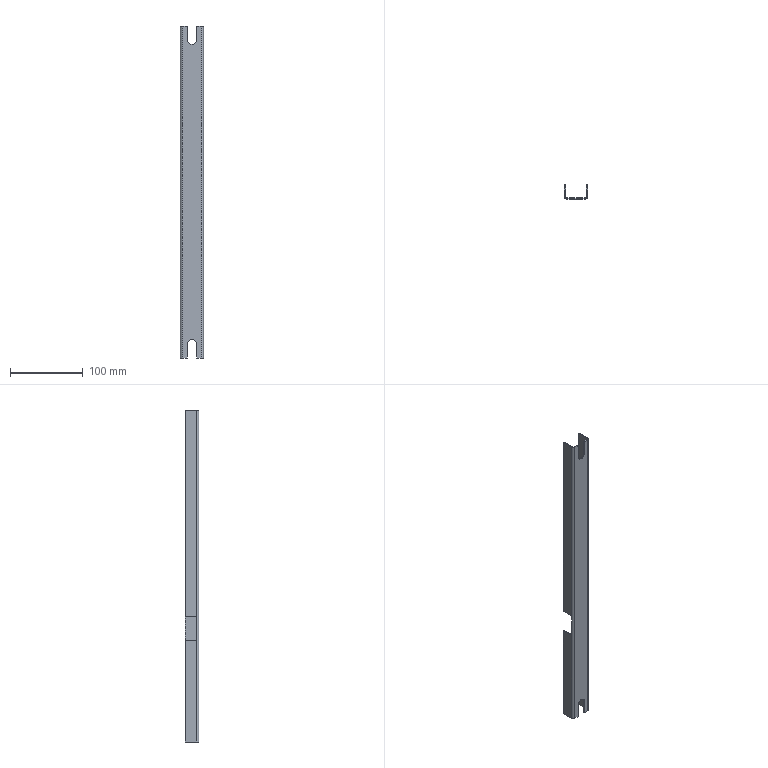Part | SolidWorks | features ICE 2, Extrusion 1, MirrorPattern 1 | 1 solid | 28 faces | box 31.75 x 19.05 x 457.2 mm | volume 42632 mm3 | plane 21 | cylinder 7 | commonest cylinder face diameters 12.7 x3 3.2 x2 6.4 x2
STEP:
#1=CARTESIAN_POINT('',(15.875,1.5,431.8));
#2=VERTEX_POINT('',#1);
#3=CARTESIAN_POINT('',(22.225,1.5,438.15));
#4=VERTEX_POINT('',#3);
#5=CARTESIAN_POINT('',(15.875,1.5,438.15));
#6=DIRECTION('',(0.,-1.,0.));
#7=DIRECTION('',(0.,0.,-1.));
#8=AXIS2_PLACEMENT_3D('',#5,#6,#7);
#9=CIRCLE('',#8,6.35);
#10=EDGE_CURVE('',#2,#4,#9,.T.);
#11=ORIENTED_EDGE('',*,*,#10,.F.);
#12=CARTESIAN_POINT('',(15.875,0.,431.8));
#13=VERTEX_POINT('',#12);
#14=CARTESIAN_POINT('',(15.875,19.05,431.8));
#15=DIRECTION('',(0.,-1.,0.));
#16=VECTOR('',#15,1000.);
#17=LINE('',#14,#16);
#18=EDGE_CURVE('',#2,#13,#17,.T.);
#19=ORIENTED_EDGE('',*,*,#18,.T.);
#20=CARTESIAN_POINT('',(22.225,0.,438.15));
#21=VERTEX_POINT('',#20);
#22=CARTESIAN_POINT('',(15.875,0.,438.15));
#23=DIRECTION('',(0.,-1.,0.));
#24=DIRECTION('',(0.,0.,-1.));
#25=AXIS2_PLACEMENT_3D('',#22,#23,#24);
#26=CIRCLE('',#25,6.35);
#27=EDGE_CURVE('',#13,#21,#26,.T.);
#28=ORIENTED_EDGE('',*,*,#27,.T.);
#29=CARTESIAN_POINT('',(22.225,19.05,438.15));
#30=DIRECTION('',(0.,-1.,0.));
#31=VECTOR('',#30,1000.);
#32=LINE('',#29,#31);
#33=EDGE_CURVE('',#4,#21,#32,.T.);
#34=ORIENTED_EDGE('',*,*,#33,.F.);
#35=EDGE_LOOP('',(#11,#19,#28,#34));
#36=FACE_OUTER_BOUND('',#35,.T.);
#37=CARTESIAN_POINT('',(15.875,19.05,438.15));
#38=DIRECTION('',(0.,-1.,0.));
#39=DIRECTION('',(0.,0.,-1.));
#40=AXIS2_PLACEMENT_3D('',#37,#38,#39);
#41=CYLINDRICAL_SURFACE('',#40,6.35);
#42=ADVANCED_FACE('',(#36),#41,.F.);
#43=CARTESIAN_POINT('',(9.525,1.5,0.));
#44=VERTEX_POINT('',#43);
#45=CARTESIAN_POINT('',(9.525,1.5,19.05));
#46=VERTEX_POINT('',#45);
#47=CARTESIAN_POINT('',(9.525,1.5,457.2));
#48=DIRECTION('',(0.,0.,1.));
#49=VECTOR('',#48,1000.);
#50=LINE('',#47,#49);
#51=EDGE_CURVE('',#44,#46,#50,.T.);
#52=ORIENTED_EDGE('',*,*,#51,.F.);
#53=CARTESIAN_POINT('',(3.1,1.5,0.));
#54=VERTEX_POINT('',#53);
#55=CARTESIAN_POINT('',(3.1,1.5,0.));
#56=DIRECTION('',(-1.,0.,0.));
#57=VECTOR('',#56,1000.);
#58=LINE('',#55,#57);
#59=EDGE_CURVE('',#44,#54,#58,.T.);
#60=ORIENTED_EDGE('',*,*,#59,.T.);
#61=CARTESIAN_POINT('',(3.1,1.5,457.2));
#62=VERTEX_POINT('',#61);
#63=CARTESIAN_POINT('',(3.1,1.5,457.2));
#64=DIRECTION('',(0.,0.,-1.));
#65=VECTOR('',#64,1000.);
#66=LINE('',#63,#65);
#67=EDGE_CURVE('',#62,#54,#66,.T.);
#68=ORIENTED_EDGE('',*,*,#67,.F.);
#69=CARTESIAN_POINT('',(9.525,1.5,457.2));
#70=VERTEX_POINT('',#69);
#71=CARTESIAN_POINT('',(3.1,1.5,457.2));
#72=DIRECTION('',(-1.,0.,0.));
#73=VECTOR('',#72,1000.);
#74=LINE('',#71,#73);
#75=EDGE_CURVE('',#70,#62,#74,.T.);
#76=ORIENTED_EDGE('',*,*,#75,.F.);
#77=CARTESIAN_POINT('',(9.525,1.5,438.15));
#78=VERTEX_POINT('',#77);
#79=CARTESIAN_POINT('',(9.525,1.5,457.2));
#80=DIRECTION('',(0.,0.,-1.));
#81=VECTOR('',#80,1000.);
#82=LINE('',#79,#81);
#83=EDGE_CURVE('',#70,#78,#82,.T.);
#84=ORIENTED_EDGE('',*,*,#83,.T.);
#85=CARTESIAN_POINT('',(15.875,1.5,438.15));
#86=DIRECTION('',(0.,-1.,0.));
#87=DIRECTION('',(0.,0.,-1.));
#88=AXIS2_PLACEMENT_3D('',#85,#86,#87);
#89=CIRCLE('',#88,6.35);
#90=EDGE_CURVE('',#78,#2,#89,.T.);
#91=ORIENTED_EDGE('',*,*,#90,.T.);
#92=ORIENTED_EDGE('',*,*,#10,.T.);
#93=CARTESIAN_POINT('',(22.225,1.5,457.2));
#94=VERTEX_POINT('',#93);
#95=CARTESIAN_POINT('',(22.225,1.5,457.2));
#96=DIRECTION('',(0.,0.,1.));
#97=VECTOR('',#96,1000.);
#98=LINE('',#95,#97);
#99=EDGE_CURVE('',#4,#94,#98,.T.);
#100=ORIENTED_EDGE('',*,*,#99,.T.);
#101=CARTESIAN_POINT('',(28.65,1.5,457.2));
#102=VERTEX_POINT('',#101);
#103=CARTESIAN_POINT('',(3.1,1.5,457.2));
#104=DIRECTION('',(-1.,0.,0.));
#105=VECTOR('',#104,1000.);
#106=LINE('',#103,#105);
#107=EDGE_CURVE('',#102,#94,#106,.T.);
#108=ORIENTED_EDGE('',*,*,#107,.F.);
#109=CARTESIAN_POINT('',(28.65,1.5,0.));
#110=VERTEX_POINT('',#109);
#111=CARTESIAN_POINT('',(28.65,1.5,457.2));
#112=DIRECTION('',(0.,0.,-1.));
#113=VECTOR('',#112,1000.);
#114=LINE('',#111,#113);
#115=EDGE_CURVE('',#102,#110,#114,.T.);
#116=ORIENTED_EDGE('',*,*,#115,.T.);
#117=CARTESIAN_POINT('',(22.225,1.5,0.));
#118=VERTEX_POINT('',#117);
#119=CARTESIAN_POINT('',(3.1,1.5,0.));
#120=DIRECTION('',(-1.,0.,0.));
#121=VECTOR('',#120,1000.);
#122=LINE('',#119,#121);
#123=EDGE_CURVE('',#110,#118,#122,.T.);
#124=ORIENTED_EDGE('',*,*,#123,.T.);
#125=CARTESIAN_POINT('',(22.225,1.5,19.05));
#126=VERTEX_POINT('',#125);
#127=CARTESIAN_POINT('',(22.225,1.5,457.2));
#128=DIRECTION('',(0.,0.,-1.));
#129=VECTOR('',#128,1000.);
#130=LINE('',#127,#129);
#131=EDGE_CURVE('',#126,#118,#130,.T.);
#132=ORIENTED_EDGE('',*,*,#131,.F.);
#133=CARTESIAN_POINT('',(15.875,1.5,19.05));
#134=DIRECTION('',(0.,1.,0.));
#135=DIRECTION('',(0.,0.,-1.));
#136=AXIS2_PLACEMENT_3D('',#133,#134,#135);
#137=CIRCLE('',#136,6.35);
#138=EDGE_CURVE('',#46,#126,#137,.T.);
#139=ORIENTED_EDGE('',*,*,#138,.F.);
#140=EDGE_LOOP('',(#52,#60,#68,#76,#84,#91,#92,#100,#108,#116,#124,#132,#139));
#141=FACE_OUTER_BOUND('',#140,.T.);
#142=CARTESIAN_POINT('',(3.1,1.5,457.2));
#143=DIRECTION('',(0.,-1.,0.));
#144=DIRECTION('',(0.,0.,-1.));
#145=AXIS2_PLACEMENT_3D('',#142,#143,#144);
#146=PLANE('',#145);
#147=ADVANCED_FACE('',(#141),#146,.F.);
#148=CARTESIAN_POINT('',(9.525,0.,0.));
#149=VERTEX_POINT('',#148);
#150=CARTESIAN_POINT('',(9.525,0.,19.05));
#151=VERTEX_POINT('',#150);
#152=CARTESIAN_POINT('',(9.525,0.,0.));
#153=DIRECTION('',(0.,0.,1.));
#154=VECTOR('',#153,1000.);
#155=LINE('',#152,#154);
#156=EDGE_CURVE('',#149,#151,#155,.T.);
#157=ORIENTED_EDGE('',*,*,#156,.T.);
#158=CARTESIAN_POINT('',(22.225,0.,19.05));
#159=VERTEX_POINT('',#158);
#160=CARTESIAN_POINT('',(15.875,0.,19.05));
#161=DIRECTION('',(0.,1.,0.));
#162=DIRECTION('',(0.,0.,1.));
#163=AXIS2_PLACEMENT_3D('',#160,#161,#162);
#164=CIRCLE('',#163,6.35);
#165=EDGE_CURVE('',#151,#159,#164,.T.);
#166=ORIENTED_EDGE('',*,*,#165,.T.);
#167=CARTESIAN_POINT('',(22.225,0.,0.));
#168=VERTEX_POINT('',#167);
#169=CARTESIAN_POINT('',(22.225,0.,0.));
#170=DIRECTION('',(0.,0.,-1.));
#171=VECTOR('',#170,1000.);
#172=LINE('',#169,#171);
#173=EDGE_CURVE('',#159,#168,#172,.T.);
#174=ORIENTED_EDGE('',*,*,#173,.T.);
#175=CARTESIAN_POINT('',(28.55,0.,0.));
#176=VERTEX_POINT('',#175);
#177=CARTESIAN_POINT('',(3.2,0.,0.));
#178=DIRECTION('',(1.,0.,0.));
#179=VECTOR('',#178,1000.);
#180=LINE('',#177,#179);
#181=EDGE_CURVE('',#168,#176,#180,.T.);
#182=ORIENTED_EDGE('',*,*,#181,.T.);
#183=CARTESIAN_POINT('',(28.55,0.,457.2));
#184=VERTEX_POINT('',#183);
#185=CARTESIAN_POINT('',(28.55,0.,457.2));
#186=DIRECTION('',(0.,0.,-1.));
#187=VECTOR('',#186,1000.);
#188=LINE('',#185,#187);
#189=EDGE_CURVE('',#184,#176,#188,.T.);
#190=ORIENTED_EDGE('',*,*,#189,.F.);
#191=CARTESIAN_POINT('',(22.225,0.,457.2));
#192=VERTEX_POINT('',#191);
#193=CARTESIAN_POINT('',(3.2,0.,457.2));
#194=DIRECTION('',(1.,0.,0.));
#195=VECTOR('',#194,1000.);
#196=LINE('',#193,#195);
#197=EDGE_CURVE('',#192,#184,#196,.T.);
#198=ORIENTED_EDGE('',*,*,#197,.F.);
#199=CARTESIAN_POINT('',(22.225,0.,457.2));
#200=DIRECTION('',(0.,0.,1.));
#201=VECTOR('',#200,1000.);
#202=LINE('',#199,#201);
#203=EDGE_CURVE('',#21,#192,#202,.T.);
#204=ORIENTED_EDGE('',*,*,#203,.F.);
#205=ORIENTED_EDGE('',*,*,#27,.F.);
#206=CARTESIAN_POINT('',(9.525,0.,438.15));
#207=VERTEX_POINT('',#206);
#208=CARTESIAN_POINT('',(15.875,0.,438.15));
#209=DIRECTION('',(0.,-1.,0.));
#210=DIRECTION('',(0.,0.,-1.));
#211=AXIS2_PLACEMENT_3D('',#208,#209,#210);
#212=CIRCLE('',#211,6.35);
#213=EDGE_CURVE('',#207,#13,#212,.T.);
#214=ORIENTED_EDGE('',*,*,#213,.F.);
#215=CARTESIAN_POINT('',(9.525,0.,457.2));
#216=VERTEX_POINT('',#215);
#217=CARTESIAN_POINT('',(9.525,0.,457.2));
#218=DIRECTION('',(0.,0.,-1.));
#219=VECTOR('',#218,1000.);
#220=LINE('',#217,#219);
#221=EDGE_CURVE('',#216,#207,#220,.T.);
#222=ORIENTED_EDGE('',*,*,#221,.F.);
#223=CARTESIAN_POINT('',(3.2,0.,457.2));
#224=VERTEX_POINT('',#223);
#225=CARTESIAN_POINT('',(3.2,0.,457.2));
#226=DIRECTION('',(1.,0.,0.));
#227=VECTOR('',#226,1000.);
#228=LINE('',#225,#227);
#229=EDGE_CURVE('',#224,#216,#228,.T.);
#230=ORIENTED_EDGE('',*,*,#229,.F.);
#231=CARTESIAN_POINT('',(3.2,0.,0.));
#232=VERTEX_POINT('',#231);
#233=CARTESIAN_POINT('',(3.2,0.,457.2));
#234=DIRECTION('',(0.,0.,-1.));
#235=VECTOR('',#234,1000.);
#236=LINE('',#233,#235);
#237=EDGE_CURVE('',#224,#232,#236,.T.);
#238=ORIENTED_EDGE('',*,*,#237,.T.);
#239=CARTESIAN_POINT('',(3.2,0.,0.));
#240=DIRECTION('',(1.,0.,0.));
#241=VECTOR('',#240,1000.);
#242=LINE('',#239,#241);
#243=EDGE_CURVE('',#232,#149,#242,.T.);
#244=ORIENTED_EDGE('',*,*,#243,.T.);
#245=EDGE_LOOP('',(#157,#166,#174,#182,#190,#198,#204,#205,#214,#222,#230,#238,#244));
#246=FACE_OUTER_BOUND('',#245,.T.);
#247=CARTESIAN_POINT('',(3.2,0.,457.2));
#248=DIRECTION('',(0.,1.,0.));
#249=DIRECTION('',(0.,0.,1.));
#250=AXIS2_PLACEMENT_3D('',#247,#248,#249);
#251=PLANE('',#250);
#252=ADVANCED_FACE('',(#246),#251,.F.);
#253=CARTESIAN_POINT('',(9.525,3.1,0.));
#254=DIRECTION('',(0.,1.,0.));
#255=VECTOR('',#254,1000.);
#256=LINE('',#253,#255);
#257=EDGE_CURVE('',#149,#44,#256,.T.);
#258=ORIENTED_EDGE('',*,*,#257,.F.);
#259=ORIENTED_EDGE('',*,*,#243,.F.);
#260=CARTESIAN_POINT('',(0.,3.2,0.));
#261=VERTEX_POINT('',#260);
#262=CARTESIAN_POINT('',(3.2,3.2,0.));
#263=DIRECTION('',(0.,0.,1.));
#264=DIRECTION('',(1.,0.,0.));
#265=AXIS2_PLACEMENT_3D('',#262,#263,#264);
#266=CIRCLE('',#265,3.2);
#267=EDGE_CURVE('',#261,#232,#266,.T.);
#268=ORIENTED_EDGE('',*,*,#267,.F.);
#269=CARTESIAN_POINT('',(0.,19.05,0.));
#270=VERTEX_POINT('',#269);
#271=CARTESIAN_POINT('',(0.,3.2,0.));
#272=DIRECTION('',(0.,-1.,0.));
#273=VECTOR('',#272,1000.);
#274=LINE('',#271,#273);
#275=EDGE_CURVE('',#270,#261,#274,.T.);
#276=ORIENTED_EDGE('',*,*,#275,.F.);
#277=CARTESIAN_POINT('',(1.5,19.05,0.));
#278=VERTEX_POINT('',#277);
#279=CARTESIAN_POINT('',(1.5,19.05,0.));
#280=DIRECTION('',(-1.,0.,0.));
#281=VECTOR('',#280,1000.);
#282=LINE('',#279,#281);
#283=EDGE_CURVE('',#278,#270,#282,.T.);
#284=ORIENTED_EDGE('',*,*,#283,.F.);
#285=CARTESIAN_POINT('',(1.5,3.1,0.));
#286=VERTEX_POINT('',#285);
#287=CARTESIAN_POINT('',(1.5,3.1,0.));
#288=DIRECTION('',(0.,1.,0.));
#289=VECTOR('',#288,1000.);
#290=LINE('',#287,#289);
#291=EDGE_CURVE('',#286,#278,#290,.T.);
#292=ORIENTED_EDGE('',*,*,#291,.F.);
#293=CARTESIAN_POINT('',(3.1,3.1,0.));
#294=DIRECTION('',(0.,0.,-1.));
#295=DIRECTION('',(-1.,0.,0.));
#296=AXIS2_PLACEMENT_3D('',#293,#294,#295);
#297=CIRCLE('',#296,1.6);
#298=EDGE_CURVE('',#54,#286,#297,.T.);
#299=ORIENTED_EDGE('',*,*,#298,.F.);
#300=ORIENTED_EDGE('',*,*,#59,.F.);
#301=EDGE_LOOP('',(#258,#259,#268,#276,#284,#292,#299,#300));
#302=FACE_OUTER_BOUND('',#301,.T.);
#303=CARTESIAN_POINT('',(28.65,3.1,0.));
#304=DIRECTION('',(0.,0.,1.));
#305=DIRECTION('',(1.,0.,0.));
#306=AXIS2_PLACEMENT_3D('',#303,#304,#305);
#307=PLANE('',#306);
#308=ADVANCED_FACE('',(#302),#307,.F.);
#309=CARTESIAN_POINT('',(22.225,3.1,0.));
#310=DIRECTION('',(0.,-1.,0.));
#311=VECTOR('',#310,1000.);
#312=LINE('',#309,#311);
#313=EDGE_CURVE('',#118,#168,#312,.T.);
#314=ORIENTED_EDGE('',*,*,#313,.F.);
#315=ORIENTED_EDGE('',*,*,#123,.F.);
#316=CARTESIAN_POINT('',(30.25,3.1,0.));
#317=VERTEX_POINT('',#316);
#318=CARTESIAN_POINT('',(28.65,3.1,0.));
#319=DIRECTION('',(0.,0.,-1.));
#320=DIRECTION('',(1.,0.,0.));
#321=AXIS2_PLACEMENT_3D('',#318,#319,#320);
#322=CIRCLE('',#321,1.6);
#323=EDGE_CURVE('',#317,#110,#322,.T.);
#324=ORIENTED_EDGE('',*,*,#323,.F.);
#325=CARTESIAN_POINT('',(30.25,19.05,0.));
#326=VERTEX_POINT('',#325);
#327=CARTESIAN_POINT('',(30.25,3.1,0.));
#328=DIRECTION('',(0.,-1.,0.));
#329=VECTOR('',#328,1000.);
#330=LINE('',#327,#329);
#331=EDGE_CURVE('',#326,#317,#330,.T.);
#332=ORIENTED_EDGE('',*,*,#331,.F.);
#333=CARTESIAN_POINT('',(31.75,19.05,0.));
#334=VERTEX_POINT('',#333);
#335=CARTESIAN_POINT('',(31.75,19.05,0.));
#336=DIRECTION('',(-1.,0.,0.));
#337=VECTOR('',#336,1000.);
#338=LINE('',#335,#337);
#339=EDGE_CURVE('',#334,#326,#338,.T.);
#340=ORIENTED_EDGE('',*,*,#339,.F.);
#341=CARTESIAN_POINT('',(31.75,3.2,0.));
#342=VERTEX_POINT('',#341);
#343=CARTESIAN_POINT('',(31.75,3.2,0.));
#344=DIRECTION('',(0.,1.,0.));
#345=VECTOR('',#344,1000.);
#346=LINE('',#343,#345);
#347=EDGE_CURVE('',#342,#334,#346,.T.);
#348=ORIENTED_EDGE('',*,*,#347,.F.);
#349=CARTESIAN_POINT('',(28.55,3.2,0.));
#350=DIRECTION('',(0.,0.,1.));
#351=DIRECTION('',(-1.,0.,0.));
#352=AXIS2_PLACEMENT_3D('',#349,#350,#351);
#353=CIRCLE('',#352,3.2);
#354=EDGE_CURVE('',#176,#342,#353,.T.);
#355=ORIENTED_EDGE('',*,*,#354,.F.);
#356=ORIENTED_EDGE('',*,*,#181,.F.);
#357=EDGE_LOOP('',(#314,#315,#324,#332,#340,#348,#355,#356));
#358=FACE_OUTER_BOUND('',#357,.T.);
#359=CARTESIAN_POINT('',(28.65,3.1,0.));
#360=DIRECTION('',(0.,0.,1.));
#361=DIRECTION('',(1.,0.,0.));
#362=AXIS2_PLACEMENT_3D('',#359,#360,#361);
#363=PLANE('',#362);
#364=ADVANCED_FACE('',(#358),#363,.F.);
#365=CARTESIAN_POINT('',(22.225,3.1,457.2));
#366=DIRECTION('',(0.,1.,0.));
#367=VECTOR('',#366,1000.);
#368=LINE('',#365,#367);
#369=EDGE_CURVE('',#192,#94,#368,.T.);
#370=ORIENTED_EDGE('',*,*,#369,.F.);
#371=ORIENTED_EDGE('',*,*,#197,.T.);
#372=CARTESIAN_POINT('',(31.75,3.2,457.2));
#373=VERTEX_POINT('',#372);
#374=CARTESIAN_POINT('',(28.55,3.2,457.2));
#375=DIRECTION('',(0.,0.,1.));
#376=DIRECTION('',(-1.,0.,0.));
#377=AXIS2_PLACEMENT_3D('',#374,#375,#376);
#378=CIRCLE('',#377,3.2);
#379=EDGE_CURVE('',#184,#373,#378,.T.);
#380=ORIENTED_EDGE('',*,*,#379,.T.);
#381=CARTESIAN_POINT('',(31.75,19.05,457.2));
#382=VERTEX_POINT('',#381);
#383=CARTESIAN_POINT('',(31.75,3.2,457.2));
#384=DIRECTION('',(0.,1.,0.));
#385=VECTOR('',#384,1000.);
#386=LINE('',#383,#385);
#387=EDGE_CURVE('',#373,#382,#386,.T.);
#388=ORIENTED_EDGE('',*,*,#387,.T.);
#389=CARTESIAN_POINT('',(30.25,19.05,457.2));
#390=VERTEX_POINT('',#389);
#391=CARTESIAN_POINT('',(31.75,19.05,457.2));
#392=DIRECTION('',(-1.,0.,0.));
#393=VECTOR('',#392,1000.);
#394=LINE('',#391,#393);
#395=EDGE_CURVE('',#382,#390,#394,.T.);
#396=ORIENTED_EDGE('',*,*,#395,.T.);
#397=CARTESIAN_POINT('',(30.25,3.1,457.2));
#398=VERTEX_POINT('',#397);
#399=CARTESIAN_POINT('',(30.25,3.1,457.2));
#400=DIRECTION('',(0.,-1.,0.));
#401=VECTOR('',#400,1000.);
#402=LINE('',#399,#401);
#403=EDGE_CURVE('',#390,#398,#402,.T.);
#404=ORIENTED_EDGE('',*,*,#403,.T.);
#405=CARTESIAN_POINT('',(28.65,3.1,457.2));
#406=DIRECTION('',(0.,0.,-1.));
#407=DIRECTION('',(1.,0.,0.));
#408=AXIS2_PLACEMENT_3D('',#405,#406,#407);
#409=CIRCLE('',#408,1.6);
#410=EDGE_CURVE('',#398,#102,#409,.T.);
#411=ORIENTED_EDGE('',*,*,#410,.T.);
#412=ORIENTED_EDGE('',*,*,#107,.T.);
#413=EDGE_LOOP('',(#370,#371,#380,#388,#396,#404,#411,#412));
#414=FACE_OUTER_BOUND('',#413,.T.);
#415=CARTESIAN_POINT('',(28.65,3.1,457.2));
#416=DIRECTION('',(0.,0.,1.));
#417=DIRECTION('',(1.,0.,0.));
#418=AXIS2_PLACEMENT_3D('',#415,#416,#417);
#419=PLANE('',#418);
#420=ADVANCED_FACE('',(#414),#419,.T.);
#421=CARTESIAN_POINT('',(1.5,19.05,457.2));
#422=VERTEX_POINT('',#421);
#423=CARTESIAN_POINT('',(1.5,19.05,172.974));
#424=VERTEX_POINT('',#423);
#425=CARTESIAN_POINT('',(1.5,19.05,457.2));
#426=DIRECTION('',(0.,0.,-1.));
#427=VECTOR('',#426,1000.);
#428=LINE('',#425,#427);
#429=EDGE_CURVE('',#422,#424,#428,.T.);
#430=ORIENTED_EDGE('',*,*,#429,.T.);
#431=CARTESIAN_POINT('',(0.,19.05,172.974));
#432=VERTEX_POINT('',#431);
#433=CARTESIAN_POINT('',(31.751,19.05,172.974));
#434=DIRECTION('',(-1.,0.,0.));
#435=VECTOR('',#434,1000.);
#436=LINE('',#433,#435);
#437=EDGE_CURVE('',#424,#432,#436,.T.);
#438=ORIENTED_EDGE('',*,*,#437,.T.);
#439=CARTESIAN_POINT('',(0.,19.05,457.2));
#440=VERTEX_POINT('',#439);
#441=CARTESIAN_POINT('',(0.,19.05,457.2));
#442=DIRECTION('',(0.,0.,-1.));
#443=VECTOR('',#442,1000.);
#444=LINE('',#441,#443);
#445=EDGE_CURVE('',#440,#432,#444,.T.);
#446=ORIENTED_EDGE('',*,*,#445,.F.);
#447=CARTESIAN_POINT('',(1.5,19.05,457.2));
#448=DIRECTION('',(-1.,0.,0.));
#449=VECTOR('',#448,1000.);
#450=LINE('',#447,#449);
#451=EDGE_CURVE('',#422,#440,#450,.T.);
#452=ORIENTED_EDGE('',*,*,#451,.F.);
#453=EDGE_LOOP('',(#430,#438,#446,#452));
#454=FACE_OUTER_BOUND('',#453,.T.);
#455=CARTESIAN_POINT('',(1.5,19.05,457.2));
#456=DIRECTION('',(0.,-1.,0.));
#457=DIRECTION('',(0.,0.,-1.));
#458=AXIS2_PLACEMENT_3D('',#455,#456,#457);
#459=PLANE('',#458);
#460=ADVANCED_FACE('',(#454),#459,.F.);
#461=ORIENTED_EDGE('',*,*,#445,.T.);
#462=CARTESIAN_POINT('',(0.,3.2,172.974));
#463=VERTEX_POINT('',#462);
#464=CARTESIAN_POINT('',(0.,19.05,172.974));
#465=DIRECTION('',(0.,1.,0.));
#466=VECTOR('',#465,1000.);
#467=LINE('',#464,#466);
#468=EDGE_CURVE('',#463,#432,#467,.T.);
#469=ORIENTED_EDGE('',*,*,#468,.F.);
#470=CARTESIAN_POINT('',(0.,3.2,457.2));
#471=VERTEX_POINT('',#470);
#472=CARTESIAN_POINT('',(0.,3.2,457.2));
#473=DIRECTION('',(0.,0.,-1.));
#474=VECTOR('',#473,1000.);
#475=LINE('',#472,#474);
#476=EDGE_CURVE('',#471,#463,#475,.T.);
#477=ORIENTED_EDGE('',*,*,#476,.F.);
#478=CARTESIAN_POINT('',(0.,3.2,457.2));
#479=DIRECTION('',(0.,-1.,0.));
#480=VECTOR('',#479,1000.);
#481=LINE('',#478,#480);
#482=EDGE_CURVE('',#440,#471,#481,.T.);
#483=ORIENTED_EDGE('',*,*,#482,.F.);
#484=EDGE_LOOP('',(#461,#469,#477,#483));
#485=FACE_OUTER_BOUND('',#484,.T.);
#486=CARTESIAN_POINT('',(0.,3.2,457.2));
#487=DIRECTION('',(1.,0.,0.));
#488=DIRECTION('',(0.,0.,-1.));
#489=AXIS2_PLACEMENT_3D('',#486,#487,#488);
#490=PLANE('',#489);
#491=ADVANCED_FACE('',(#485),#490,.F.);
#492=ORIENTED_EDGE('',*,*,#339,.T.);
#493=CARTESIAN_POINT('',(30.25,19.05,457.2));
#494=DIRECTION('',(0.,0.,-1.));
#495=VECTOR('',#494,1000.);
#496=LINE('',#493,#495);
#497=EDGE_CURVE('',#390,#326,#496,.T.);
#498=ORIENTED_EDGE('',*,*,#497,.F.);
#499=ORIENTED_EDGE('',*,*,#395,.F.);
#500=CARTESIAN_POINT('',(31.75,19.05,457.2));
#501=DIRECTION('',(0.,0.,-1.));
#502=VECTOR('',#501,1000.);
#503=LINE('',#500,#502);
#504=EDGE_CURVE('',#382,#334,#503,.T.);
#505=ORIENTED_EDGE('',*,*,#504,.T.);
#506=EDGE_LOOP('',(#492,#498,#499,#505));
#507=FACE_OUTER_BOUND('',#506,.T.);
#508=CARTESIAN_POINT('',(31.75,19.05,457.2));
#509=DIRECTION('',(0.,-1.,0.));
#510=DIRECTION('',(0.,0.,-1.));
#511=AXIS2_PLACEMENT_3D('',#508,#509,#510);
#512=PLANE('',#511);
#513=ADVANCED_FACE('',(#507),#512,.F.);
#514=ORIENTED_EDGE('',*,*,#331,.T.);
#515=CARTESIAN_POINT('',(30.25,3.1,457.2));
#516=DIRECTION('',(0.,0.,-1.));
#517=VECTOR('',#516,1000.);
#518=LINE('',#515,#517);
#519=EDGE_CURVE('',#398,#317,#518,.T.);
#520=ORIENTED_EDGE('',*,*,#519,.F.);
#521=ORIENTED_EDGE('',*,*,#403,.F.);
#522=ORIENTED_EDGE('',*,*,#497,.T.);
#523=EDGE_LOOP('',(#514,#520,#521,#522));
#524=FACE_OUTER_BOUND('',#523,.T.);
#525=CARTESIAN_POINT('',(30.25,3.1,457.2));
#526=DIRECTION('',(1.,0.,0.));
#527=DIRECTION('',(0.,1.,0.));
#528=AXIS2_PLACEMENT_3D('',#525,#526,#527);
#529=PLANE('',#528);
#530=ADVANCED_FACE('',(#524),#529,.F.);
#531=ORIENTED_EDGE('',*,*,#323,.T.);
#532=ORIENTED_EDGE('',*,*,#115,.F.);
#533=ORIENTED_EDGE('',*,*,#410,.F.);
#534=ORIENTED_EDGE('',*,*,#519,.T.);
#535=EDGE_LOOP('',(#531,#532,#533,#534));
#536=FACE_OUTER_BOUND('',#535,.T.);
#537=CARTESIAN_POINT('',(28.65,3.1,457.2));
#538=DIRECTION('',(0.,0.,-1.));
#539=DIRECTION('',(-1.,0.,0.));
#540=AXIS2_PLACEMENT_3D('',#537,#538,#539);
#541=CYLINDRICAL_SURFACE('',#540,1.6);
#542=ADVANCED_FACE('',(#536),#541,.F.);
#543=ORIENTED_EDGE('',*,*,#298,.T.);
#544=CARTESIAN_POINT('',(1.5,3.1,457.2));
#545=VERTEX_POINT('',#544);
#546=CARTESIAN_POINT('',(1.5,3.1,457.2));
#547=DIRECTION('',(0.,0.,-1.));
#548=VECTOR('',#547,1000.);
#549=LINE('',#546,#548);
#550=EDGE_CURVE('',#545,#286,#549,.T.);
#551=ORIENTED_EDGE('',*,*,#550,.F.);
#552=CARTESIAN_POINT('',(3.1,3.1,457.2));
#553=DIRECTION('',(0.,0.,-1.));
#554=DIRECTION('',(-1.,0.,0.));
#555=AXIS2_PLACEMENT_3D('',#552,#553,#554);
#556=CIRCLE('',#555,1.6);
#557=EDGE_CURVE('',#62,#545,#556,.T.);
#558=ORIENTED_EDGE('',*,*,#557,.F.);
#559=ORIENTED_EDGE('',*,*,#67,.T.);
#560=EDGE_LOOP('',(#543,#551,#558,#559));
#561=FACE_OUTER_BOUND('',#560,.T.);
#562=CARTESIAN_POINT('',(3.1,3.1,457.2));
#563=DIRECTION('',(0.,0.,-1.));
#564=DIRECTION('',(-1.,0.,0.));
#565=AXIS2_PLACEMENT_3D('',#562,#563,#564);
#566=CYLINDRICAL_SURFACE('',#565,1.6);
#567=ADVANCED_FACE('',(#561),#566,.F.);
#568=CARTESIAN_POINT('',(1.5,3.2,172.974));
#569=VERTEX_POINT('',#568);
#570=CARTESIAN_POINT('',(1.5,3.2,139.7));
#571=VERTEX_POINT('',#570);
#572=CARTESIAN_POINT('',(1.5,3.2,172.974));
#573=DIRECTION('',(0.,0.,-1.));
#574=VECTOR('',#573,1000.);
#575=LINE('',#572,#574);
#576=EDGE_CURVE('',#569,#571,#575,.T.);
#577=ORIENTED_EDGE('',*,*,#576,.F.);
#578=CARTESIAN_POINT('',(1.5,19.05,172.974));
#579=DIRECTION('',(0.,-1.,0.));
#580=VECTOR('',#579,1000.);
#581=LINE('',#578,#580);
#582=EDGE_CURVE('',#424,#569,#581,.T.);
#583=ORIENTED_EDGE('',*,*,#582,.F.);
#584=ORIENTED_EDGE('',*,*,#429,.F.);
#585=CARTESIAN_POINT('',(1.5,3.1,457.2));
#586=DIRECTION('',(0.,1.,0.));
#587=VECTOR('',#586,1000.);
#588=LINE('',#585,#587);
#589=EDGE_CURVE('',#545,#422,#588,.T.);
#590=ORIENTED_EDGE('',*,*,#589,.F.);
#591=ORIENTED_EDGE('',*,*,#550,.T.);
#592=ORIENTED_EDGE('',*,*,#291,.T.);
#593=CARTESIAN_POINT('',(1.5,19.05,139.7));
#594=VERTEX_POINT('',#593);
#595=CARTESIAN_POINT('',(1.5,19.05,457.2));
#596=DIRECTION('',(0.,0.,-1.));
#597=VECTOR('',#596,1000.);
#598=LINE('',#595,#597);
#599=EDGE_CURVE('',#594,#278,#598,.T.);
#600=ORIENTED_EDGE('',*,*,#599,.F.);
#601=CARTESIAN_POINT('',(1.5,19.05,139.7));
#602=DIRECTION('',(0.,1.,0.));
#603=VECTOR('',#602,1000.);
#604=LINE('',#601,#603);
#605=EDGE_CURVE('',#571,#594,#604,.T.);
#606=ORIENTED_EDGE('',*,*,#605,.F.);
#607=EDGE_LOOP('',(#577,#583,#584,#590,#591,#592,#600,#606));
#608=FACE_OUTER_BOUND('',#607,.T.);
#609=CARTESIAN_POINT('',(1.5,3.1,457.2));
#610=DIRECTION('',(-1.,0.,0.));
#611=DIRECTION('',(0.,-1.,0.));
#612=AXIS2_PLACEMENT_3D('',#609,#610,#611);
#613=PLANE('',#612);
#614=ADVANCED_FACE('',(#608),#613,.F.);
#615=CARTESIAN_POINT('',(0.,19.05,139.7));
#616=VERTEX_POINT('',#615);
#617=CARTESIAN_POINT('',(0.,19.05,457.2));
#618=DIRECTION('',(0.,0.,-1.));
#619=VECTOR('',#618,1000.);
#620=LINE('',#617,#619);
#621=EDGE_CURVE('',#616,#270,#620,.T.);
#622=ORIENTED_EDGE('',*,*,#621,.F.);
#623=CARTESIAN_POINT('',(31.751,19.05,139.7));
#624=DIRECTION('',(-1.,0.,0.));
#625=VECTOR('',#624,1000.);
#626=LINE('',#623,#625);
#627=EDGE_CURVE('',#594,#616,#626,.T.);
#628=ORIENTED_EDGE('',*,*,#627,.F.);
#629=ORIENTED_EDGE('',*,*,#599,.T.);
#630=ORIENTED_EDGE('',*,*,#283,.T.);
#631=EDGE_LOOP('',(#622,#628,#629,#630));
#632=FACE_OUTER_BOUND('',#631,.T.);
#633=CARTESIAN_POINT('',(1.5,19.05,457.2));
#634=DIRECTION('',(0.,-1.,0.));
#635=DIRECTION('',(0.,0.,-1.));
#636=AXIS2_PLACEMENT_3D('',#633,#634,#635);
#637=PLANE('',#636);
#638=ADVANCED_FACE('',(#632),#637,.F.);
#639=CARTESIAN_POINT('',(0.,3.2,139.7));
#640=VERTEX_POINT('',#639);
#641=CARTESIAN_POINT('',(0.,3.2,457.2));
#642=DIRECTION('',(0.,0.,-1.));
#643=VECTOR('',#642,1000.);
#644=LINE('',#641,#643);
#645=EDGE_CURVE('',#640,#261,#644,.T.);
#646=ORIENTED_EDGE('',*,*,#645,.F.);
#647=CARTESIAN_POINT('',(0.,19.05,139.7));
#648=DIRECTION('',(0.,-1.,0.));
#649=VECTOR('',#648,1000.);
#650=LINE('',#647,#649);
#651=EDGE_CURVE('',#616,#640,#650,.T.);
#652=ORIENTED_EDGE('',*,*,#651,.F.);
#653=ORIENTED_EDGE('',*,*,#621,.T.);
#654=ORIENTED_EDGE('',*,*,#275,.T.);
#655=EDGE_LOOP('',(#646,#652,#653,#654));
#656=FACE_OUTER_BOUND('',#655,.T.);
#657=CARTESIAN_POINT('',(0.,3.2,457.2));
#658=DIRECTION('',(1.,0.,0.));
#659=DIRECTION('',(0.,0.,-1.));
#660=AXIS2_PLACEMENT_3D('',#657,#658,#659);
#661=PLANE('',#660);
#662=ADVANCED_FACE('',(#656),#661,.F.);
#663=ORIENTED_EDGE('',*,*,#267,.T.);
#664=ORIENTED_EDGE('',*,*,#237,.F.);
#665=CARTESIAN_POINT('',(3.2,3.2,457.2));
#666=DIRECTION('',(0.,0.,1.));
#667=DIRECTION('',(1.,0.,0.));
#668=AXIS2_PLACEMENT_3D('',#665,#666,#667);
#669=CIRCLE('',#668,3.2);
#670=EDGE_CURVE('',#471,#224,#669,.T.);
#671=ORIENTED_EDGE('',*,*,#670,.F.);
#672=ORIENTED_EDGE('',*,*,#476,.T.);
#673=CARTESIAN_POINT('',(0.,3.2,172.974));
#674=DIRECTION('',(0.,0.,1.));
#675=VECTOR('',#674,1000.);
#676=LINE('',#673,#675);
#677=EDGE_CURVE('',#640,#463,#676,.T.);
#678=ORIENTED_EDGE('',*,*,#677,.F.);
#679=ORIENTED_EDGE('',*,*,#645,.T.);
#680=EDGE_LOOP('',(#663,#664,#671,#672,#678,#679));
#681=FACE_OUTER_BOUND('',#680,.T.);
#682=CARTESIAN_POINT('',(3.2,3.2,457.2));
#683=DIRECTION('',(0.,0.,-1.));
#684=DIRECTION('',(-1.,0.,0.));
#685=AXIS2_PLACEMENT_3D('',#682,#683,#684);
#686=CYLINDRICAL_SURFACE('',#685,3.2);
#687=ADVANCED_FACE('',(#681),#686,.T.);
#688=ORIENTED_EDGE('',*,*,#354,.T.);
#689=CARTESIAN_POINT('',(31.75,3.2,457.2));
#690=DIRECTION('',(0.,0.,-1.));
#691=VECTOR('',#690,1000.);
#692=LINE('',#689,#691);
#693=EDGE_CURVE('',#373,#342,#692,.T.);
#694=ORIENTED_EDGE('',*,*,#693,.F.);
#695=ORIENTED_EDGE('',*,*,#379,.F.);
#696=ORIENTED_EDGE('',*,*,#189,.T.);
#697=EDGE_LOOP('',(#688,#694,#695,#696));
#698=FACE_OUTER_BOUND('',#697,.T.);
#699=CARTESIAN_POINT('',(28.55,3.2,457.2));
#700=DIRECTION('',(0.,0.,-1.));
#701=DIRECTION('',(-1.,0.,0.));
#702=AXIS2_PLACEMENT_3D('',#699,#700,#701);
#703=CYLINDRICAL_SURFACE('',#702,3.2);
#704=ADVANCED_FACE('',(#698),#703,.T.);
#705=ORIENTED_EDGE('',*,*,#347,.T.);
#706=ORIENTED_EDGE('',*,*,#504,.F.);
#707=ORIENTED_EDGE('',*,*,#387,.F.);
#708=ORIENTED_EDGE('',*,*,#693,.T.);
#709=EDGE_LOOP('',(#705,#706,#707,#708));
#710=FACE_OUTER_BOUND('',#709,.T.);
#711=CARTESIAN_POINT('',(31.75,3.2,457.2));
#712=DIRECTION('',(-1.,0.,0.));
#713=DIRECTION('',(0.,0.,1.));
#714=AXIS2_PLACEMENT_3D('',#711,#712,#713);
#715=PLANE('',#714);
#716=ADVANCED_FACE('',(#710),#715,.F.);
#717=CARTESIAN_POINT('',(9.525,3.1,457.2));
#718=DIRECTION('',(0.,-1.,0.));
#719=VECTOR('',#718,1000.);
#720=LINE('',#717,#719);
#721=EDGE_CURVE('',#70,#216,#720,.T.);
#722=ORIENTED_EDGE('',*,*,#721,.F.);
#723=ORIENTED_EDGE('',*,*,#75,.T.);
#724=ORIENTED_EDGE('',*,*,#557,.T.);
#725=ORIENTED_EDGE('',*,*,#589,.T.);
#726=ORIENTED_EDGE('',*,*,#451,.T.);
#727=ORIENTED_EDGE('',*,*,#482,.T.);
#728=ORIENTED_EDGE('',*,*,#670,.T.);
#729=ORIENTED_EDGE('',*,*,#229,.T.);
#730=EDGE_LOOP('',(#722,#723,#724,#725,#726,#727,#728,#729));
#731=FACE_OUTER_BOUND('',#730,.T.);
#732=CARTESIAN_POINT('',(28.65,3.1,457.2));
#733=DIRECTION('',(0.,0.,1.));
#734=DIRECTION('',(1.,0.,0.));
#735=AXIS2_PLACEMENT_3D('',#732,#733,#734);
#736=PLANE('',#735);
#737=ADVANCED_FACE('',(#731),#736,.T.);
#738=ORIENTED_EDGE('',*,*,#582,.T.);
#739=CARTESIAN_POINT('',(31.751,3.2,172.974));
#740=DIRECTION('',(-1.,0.,0.));
#741=VECTOR('',#740,1000.);
#742=LINE('',#739,#741);
#743=EDGE_CURVE('',#569,#463,#742,.T.);
#744=ORIENTED_EDGE('',*,*,#743,.T.);
#745=ORIENTED_EDGE('',*,*,#468,.T.);
#746=ORIENTED_EDGE('',*,*,#437,.F.);
#747=EDGE_LOOP('',(#738,#744,#745,#746));
#748=FACE_OUTER_BOUND('',#747,.T.);
#749=CARTESIAN_POINT('',(31.751,19.05,172.974));
#750=DIRECTION('',(0.,0.,1.));
#751=DIRECTION('',(1.,0.,0.));
#752=AXIS2_PLACEMENT_3D('',#749,#750,#751);
#753=PLANE('',#752);
#754=ADVANCED_FACE('',(#748),#753,.F.);
#755=ORIENTED_EDGE('',*,*,#576,.T.);
#756=CARTESIAN_POINT('',(31.751,3.2,139.7));
#757=DIRECTION('',(-1.,0.,0.));
#758=VECTOR('',#757,1000.);
#759=LINE('',#756,#758);
#760=EDGE_CURVE('',#571,#640,#759,.T.);
#761=ORIENTED_EDGE('',*,*,#760,.T.);
#762=ORIENTED_EDGE('',*,*,#677,.T.);
#763=ORIENTED_EDGE('',*,*,#743,.F.);
#764=EDGE_LOOP('',(#755,#761,#762,#763));
#765=FACE_OUTER_BOUND('',#764,.T.);
#766=CARTESIAN_POINT('',(31.751,3.2,172.974));
#767=DIRECTION('',(0.,-1.,0.));
#768=DIRECTION('',(0.,0.,-1.));
#769=AXIS2_PLACEMENT_3D('',#766,#767,#768);
#770=PLANE('',#769);
#771=ADVANCED_FACE('',(#765),#770,.F.);
#772=ORIENTED_EDGE('',*,*,#605,.T.);
#773=ORIENTED_EDGE('',*,*,#627,.T.);
#774=ORIENTED_EDGE('',*,*,#651,.T.);
#775=ORIENTED_EDGE('',*,*,#760,.F.);
#776=EDGE_LOOP('',(#772,#773,#774,#775));
#777=FACE_OUTER_BOUND('',#776,.T.);
#778=CARTESIAN_POINT('',(31.751,19.05,139.7));
#779=DIRECTION('',(0.,0.,-1.));
#780=DIRECTION('',(-1.,0.,0.));
#781=AXIS2_PLACEMENT_3D('',#778,#779,#780);
#782=PLANE('',#781);
#783=ADVANCED_FACE('',(#777),#782,.F.);
#784=ORIENTED_EDGE('',*,*,#18,.F.);
#785=ORIENTED_EDGE('',*,*,#90,.F.);
#786=CARTESIAN_POINT('',(9.525,19.05,438.15));
#787=DIRECTION('',(0.,-1.,0.));
#788=VECTOR('',#787,1000.);
#789=LINE('',#786,#788);
#790=EDGE_CURVE('',#78,#207,#789,.T.);
#791=ORIENTED_EDGE('',*,*,#790,.T.);
#792=ORIENTED_EDGE('',*,*,#213,.T.);
#793=EDGE_LOOP('',(#784,#785,#791,#792));
#794=FACE_OUTER_BOUND('',#793,.T.);
#795=CARTESIAN_POINT('',(15.875,19.05,438.15));
#796=DIRECTION('',(0.,-1.,0.));
#797=DIRECTION('',(0.,0.,-1.));
#798=AXIS2_PLACEMENT_3D('',#795,#796,#797);
#799=CYLINDRICAL_SURFACE('',#798,6.35);
#800=ADVANCED_FACE('',(#794),#799,.F.);
#801=ORIENTED_EDGE('',*,*,#33,.T.);
#802=ORIENTED_EDGE('',*,*,#203,.T.);
#803=ORIENTED_EDGE('',*,*,#369,.T.);
#804=ORIENTED_EDGE('',*,*,#99,.F.);
#805=EDGE_LOOP('',(#801,#802,#803,#804));
#806=FACE_OUTER_BOUND('',#805,.T.);
#807=CARTESIAN_POINT('',(22.225,19.05,457.2));
#808=DIRECTION('',(1.,0.,0.));
#809=DIRECTION('',(0.,0.,-1.));
#810=AXIS2_PLACEMENT_3D('',#807,#808,#809);
#811=PLANE('',#810);
#812=ADVANCED_FACE('',(#806),#811,.F.);
#813=ORIENTED_EDGE('',*,*,#721,.T.);
#814=ORIENTED_EDGE('',*,*,#221,.T.);
#815=ORIENTED_EDGE('',*,*,#790,.F.);
#816=ORIENTED_EDGE('',*,*,#83,.F.);
#817=EDGE_LOOP('',(#813,#814,#815,#816));
#818=FACE_OUTER_BOUND('',#817,.T.);
#819=CARTESIAN_POINT('',(9.525,19.05,457.2));
#820=DIRECTION('',(-1.,0.,0.));
#821=DIRECTION('',(0.,0.,1.));
#822=AXIS2_PLACEMENT_3D('',#819,#820,#821);
#823=PLANE('',#822);
#824=ADVANCED_FACE('',(#818),#823,.F.);
#825=ORIENTED_EDGE('',*,*,#138,.T.);
#826=CARTESIAN_POINT('',(22.225,19.05,19.05));
#827=DIRECTION('',(0.,-1.,0.));
#828=VECTOR('',#827,1000.);
#829=LINE('',#826,#828);
#830=EDGE_CURVE('',#126,#159,#829,.T.);
#831=ORIENTED_EDGE('',*,*,#830,.T.);
#832=ORIENTED_EDGE('',*,*,#165,.F.);
#833=CARTESIAN_POINT('',(9.525,19.05,19.05));
#834=DIRECTION('',(0.,-1.,0.));
#835=VECTOR('',#834,1000.);
#836=LINE('',#833,#835);
#837=EDGE_CURVE('',#46,#151,#836,.T.);
#838=ORIENTED_EDGE('',*,*,#837,.F.);
#839=EDGE_LOOP('',(#825,#831,#832,#838));
#840=FACE_OUTER_BOUND('',#839,.T.);
#841=CARTESIAN_POINT('',(15.875,19.05,19.05));
#842=DIRECTION('',(0.,-1.,0.));
#843=DIRECTION('',(0.,0.,-1.));
#844=AXIS2_PLACEMENT_3D('',#841,#842,#843);
#845=CYLINDRICAL_SURFACE('',#844,6.35);
#846=ADVANCED_FACE('',(#840),#845,.F.);
#847=ORIENTED_EDGE('',*,*,#51,.T.);
#848=ORIENTED_EDGE('',*,*,#837,.T.);
#849=ORIENTED_EDGE('',*,*,#156,.F.);
#850=ORIENTED_EDGE('',*,*,#257,.T.);
#851=EDGE_LOOP('',(#847,#848,#849,#850));
#852=FACE_OUTER_BOUND('',#851,.T.);
#853=CARTESIAN_POINT('',(9.525,19.05,0.));
#854=DIRECTION('',(1.,0.,0.));
#855=DIRECTION('',(0.,0.,-1.));
#856=AXIS2_PLACEMENT_3D('',#853,#854,#855);
#857=PLANE('',#856);
#858=ADVANCED_FACE('',(#852),#857,.T.);
#859=ORIENTED_EDGE('',*,*,#131,.T.);
#860=ORIENTED_EDGE('',*,*,#313,.T.);
#861=ORIENTED_EDGE('',*,*,#173,.F.);
#862=ORIENTED_EDGE('',*,*,#830,.F.);
#863=EDGE_LOOP('',(#859,#860,#861,#862));
#864=FACE_OUTER_BOUND('',#863,.T.);
#865=CARTESIAN_POINT('',(22.225,19.05,0.));
#866=DIRECTION('',(-1.,0.,0.));
#867=DIRECTION('',(0.,0.,1.));
#868=AXIS2_PLACEMENT_3D('',#865,#866,#867);
#869=PLANE('',#868);
#870=ADVANCED_FACE('',(#864),#869,.T.);
#871=CLOSED_SHELL('',(#42,#147,#252,#308,#364,#420,#460,#491,#513,#530,#542,#567,#614,#638,#662,#687,#704,#716,#737,#754,#771,#783,#800,#812,#824,#846,#858,#870));
#872=MANIFOLD_SOLID_BREP('',#871);
#873=CARTESIAN_POINT('',(0.,0.,0.));
#874=DIRECTION('',(0.,0.,1.));
#875=DIRECTION('',(1.,0.,0.));
#876=AXIS2_PLACEMENT_3D('',#873,#874,#875);
#877=(LENGTH_UNIT()NAMED_UNIT(*)SI_UNIT(.MILLI.,.METRE.));
#878=UNCERTAINTY_MEASURE_WITH_UNIT(LENGTH_MEASURE(0.00001),#877,'','');
#879=(NAMED_UNIT(*)PLANE_ANGLE_UNIT()SI_UNIT($,.RADIAN.));
#880=(NAMED_UNIT(*)SI_UNIT($,.STERADIAN.)SOLID_ANGLE_UNIT());
#881=(GEOMETRIC_REPRESENTATION_CONTEXT(3)GLOBAL_UNCERTAINTY_ASSIGNED_CONTEXT((#878))GLOBAL_UNIT_ASSIGNED_CONTEXT((#877,#879,#880))REPRESENTATION_CONTEXT('',''));
#882=ADVANCED_BREP_SHAPE_REPRESENTATION('',(#872,#876),#881);